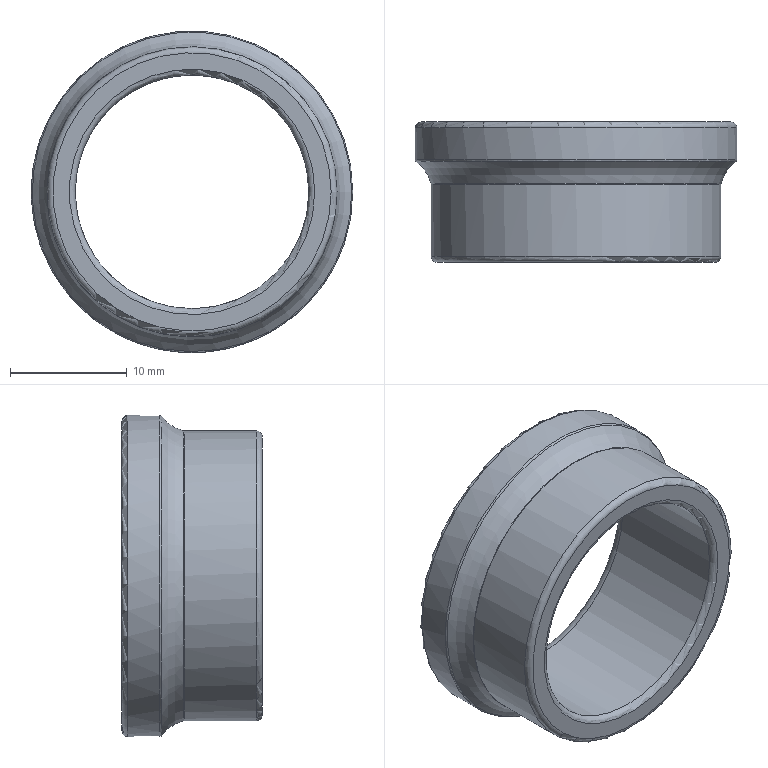Part | STEP file | BK-20_id1254_x_t | 1 solid | 12 faces | box 27.5 x 12 x 27.5 mm | volume 2449 mm3 | torus 7 | cylinder 3 | plane 2 | commonest cylinder face diameters 20 x1 24.8 x1 27.5 x1
STEP:
#1=CARTESIAN_POINT('',(0.,0.,0.));
#2=DIRECTION('',(0.,0.,1.));
#3=DIRECTION('',(1.,0.,0.));
#4=AXIS2_PLACEMENT_3D('',#1,#2,#3);
#5=CARTESIAN_POINT('',(-260.083,526.527,-176.266));
#6=VERTEX_POINT('',#5);
#7=CARTESIAN_POINT('',(-254.834,526.527,-165.5));
#8=VERTEX_POINT('',#7);
#9=CARTESIAN_POINT('',(-268.5,526.527,-165.5));
#10=DIRECTION('',(0.,1.,0.));
#11=DIRECTION('',(0.6159,0.,-0.7878));
#12=AXIS2_PLACEMENT_3D('',#9,#10,#11);
#13=CIRCLE('',#12,13.666);
#14=CARTESIAN_POINT('',(-268.5,523.936,-165.5));
#15=DIRECTION('',(0.,-1.,0.));
#16=DIRECTION('',(1.,0.,0.));
#17=AXIS2_PLACEMENT_3D('',#14,#15,#16);
#18=TOROIDAL_SURFACE('',#17,15.5,3.175);
#19=CARTESIAN_POINT('',(11.659,4.096));
#20=DIRECTION('',(-1.,0.));
#21=VECTOR('',#20,1.);
#22=LINE('',#19,#21);
#23=(GEOMETRIC_REPRESENTATION_CONTEXT(2)PARAMETRIC_REPRESENTATION_CONTEXT()REPRESENTATION_CONTEXT('',''));
#24=DEFINITIONAL_REPRESENTATION('',(#22),#23);
#25=PCURVE('',#18,#24);
#26=CARTESIAN_POINT('',(-268.5,526.69,-165.5));
#27=DIRECTION('',(0.,-1.,0.));
#28=DIRECTION('',(1.,0.,0.));
#29=AXIS2_PLACEMENT_3D('',#26,#27,#28);
#30=TOROIDAL_SURFACE('',#29,13.55,0.2);
#31=CARTESIAN_POINT('',(5.376,7.238));
#32=DIRECTION('',(-1.,0.));
#33=VECTOR('',#32,1.);
#34=LINE('',#31,#33);
#35=(GEOMETRIC_REPRESENTATION_CONTEXT(2)PARAMETRIC_REPRESENTATION_CONTEXT()REPRESENTATION_CONTEXT('',''));
#36=DEFINITIONAL_REPRESENTATION('',(#34),#35);
#37=PCURVE('',#30,#36);
#38=SURFACE_CURVE('',#13,(#25,#37),.PCURVE_S1.);
#39=EDGE_CURVE('',#6,#8,#38,.T.);
#40=ORIENTED_EDGE('',*,*,#39,.T.);
#41=CARTESIAN_POINT('',(-268.5,526.527,-165.5));
#42=DIRECTION('',(0.,1.,0.));
#43=DIRECTION('',(0.6159,0.,-0.7878));
#44=AXIS2_PLACEMENT_3D('',#41,#42,#43);
#45=CIRCLE('',#44,13.666);
#46=CARTESIAN_POINT('',(11.659,4.096));
#47=DIRECTION('',(-1.,0.));
#48=VECTOR('',#47,1.);
#49=LINE('',#46,#48);
#50=(GEOMETRIC_REPRESENTATION_CONTEXT(2)PARAMETRIC_REPRESENTATION_CONTEXT()REPRESENTATION_CONTEXT('',''));
#51=DEFINITIONAL_REPRESENTATION('',(#49),#50);
#52=PCURVE('',#18,#51);
#53=CARTESIAN_POINT('',(11.659,7.238));
#54=DIRECTION('',(-1.,0.));
#55=VECTOR('',#54,1.);
#56=LINE('',#53,#55);
#57=(GEOMETRIC_REPRESENTATION_CONTEXT(2)PARAMETRIC_REPRESENTATION_CONTEXT()REPRESENTATION_CONTEXT('',''));
#58=DEFINITIONAL_REPRESENTATION('',(#56),#57);
#59=PCURVE('',#30,#58);
#60=SURFACE_CURVE('',#45,(#52,#59),.PCURVE_S1.);
#61=EDGE_CURVE('',#8,#6,#60,.T.);
#62=ORIENTED_EDGE('',*,*,#61,.T.);
#63=CARTESIAN_POINT('',(-260.86,524.644,-175.273));
#64=VERTEX_POINT('',#63);
#65=CARTESIAN_POINT('',(-260.86,524.644,-175.273));
#66=CARTESIAN_POINT('',(-260.806,525.022,-175.341));
#67=CARTESIAN_POINT('',(-260.719,525.386,-175.453));
#68=CARTESIAN_POINT('',(-260.6,525.725,-175.605));
#69=CARTESIAN_POINT('',(-260.452,526.034,-175.794));
#70=CARTESIAN_POINT('',(-260.278,526.303,-176.017));
#71=CARTESIAN_POINT('',(-260.083,526.527,-176.266));
#72=(BOUNDED_CURVE()B_SPLINE_CURVE(6,(#65,#66,#67,#68,#69,#70,#71),.UNSPECIFIED.,.F.,.F.)B_SPLINE_CURVE_WITH_KNOTS((7,7),(3.367,4.096),.PIECEWISE_BEZIER_KNOTS.)CURVE()GEOMETRIC_REPRESENTATION_ITEM()RATIONAL_B_SPLINE_CURVE((1.007,1.002,0.9996,0.9987,0.9996,1.002,1.007))REPRESENTATION_ITEM(''));
#73=CARTESIAN_POINT('',(5.376,0.));
#74=DIRECTION('',(0.,1.));
#75=VECTOR('',#74,1.);
#76=LINE('',#73,#75);
#77=(GEOMETRIC_REPRESENTATION_CONTEXT(2)PARAMETRIC_REPRESENTATION_CONTEXT()REPRESENTATION_CONTEXT('',''));
#78=DEFINITIONAL_REPRESENTATION('',(#76),#77);
#79=PCURVE('',#18,#78);
#80=CARTESIAN_POINT('',(11.659,0.));
#81=DIRECTION('',(0.,1.));
#82=VECTOR('',#81,1.);
#83=LINE('',#80,#82);
#84=(GEOMETRIC_REPRESENTATION_CONTEXT(2)PARAMETRIC_REPRESENTATION_CONTEXT()REPRESENTATION_CONTEXT('',''));
#85=DEFINITIONAL_REPRESENTATION('',(#83),#84);
#86=PCURVE('',#18,#85);
#87=SEAM_CURVE('',#72,(#79,#86),.PCURVE_S1.);
#88=EDGE_CURVE('',#64,#6,#87,.T.);
#89=ORIENTED_EDGE('',*,*,#88,.F.);
#90=CARTESIAN_POINT('',(-256.095,524.644,-165.5));
#91=VERTEX_POINT('',#90);
#92=CARTESIAN_POINT('',(-268.5,524.644,-165.5));
#93=DIRECTION('',(0.,1.,0.));
#94=DIRECTION('',(-0.6159,0.,0.7878));
#95=AXIS2_PLACEMENT_3D('',#92,#93,#94);
#96=CIRCLE('',#95,12.405);
#97=CARTESIAN_POINT('',(8.518,3.367));
#98=DIRECTION('',(-1.,0.));
#99=VECTOR('',#98,1.);
#100=LINE('',#97,#99);
#101=(GEOMETRIC_REPRESENTATION_CONTEXT(2)PARAMETRIC_REPRESENTATION_CONTEXT()REPRESENTATION_CONTEXT('',''));
#102=DEFINITIONAL_REPRESENTATION('',(#100),#101);
#103=PCURVE('',#18,#102);
#104=CARTESIAN_POINT('',(-268.5,524.599,-165.5));
#105=DIRECTION('',(0.,-1.,0.));
#106=DIRECTION('',(1.,0.,0.));
#107=AXIS2_PLACEMENT_3D('',#104,#105,#106);
#108=TOROIDAL_SURFACE('',#107,12.6,0.2);
#109=CARTESIAN_POINT('',(8.518,3.367));
#110=DIRECTION('',(-1.,0.));
#111=VECTOR('',#110,1.);
#112=LINE('',#109,#111);
#113=(GEOMETRIC_REPRESENTATION_CONTEXT(2)PARAMETRIC_REPRESENTATION_CONTEXT()REPRESENTATION_CONTEXT('',''));
#114=DEFINITIONAL_REPRESENTATION('',(#112),#113);
#115=PCURVE('',#108,#114);
#116=SURFACE_CURVE('',#96,(#103,#115),.PCURVE_S1.);
#117=EDGE_CURVE('',#91,#64,#116,.T.);
#118=ORIENTED_EDGE('',*,*,#117,.F.);
#119=CARTESIAN_POINT('',(-276.14,524.644,-155.727));
#120=VERTEX_POINT('',#119);
#121=CARTESIAN_POINT('',(-268.5,524.644,-165.5));
#122=DIRECTION('',(0.,1.,0.));
#123=DIRECTION('',(-0.6159,0.,0.7878));
#124=AXIS2_PLACEMENT_3D('',#121,#122,#123);
#125=CIRCLE('',#124,12.405);
#126=CARTESIAN_POINT('',(8.518,3.367));
#127=DIRECTION('',(-1.,0.));
#128=VECTOR('',#127,1.);
#129=LINE('',#126,#128);
#130=(GEOMETRIC_REPRESENTATION_CONTEXT(2)PARAMETRIC_REPRESENTATION_CONTEXT()REPRESENTATION_CONTEXT('',''));
#131=DEFINITIONAL_REPRESENTATION('',(#129),#130);
#132=PCURVE('',#18,#131);
#133=CARTESIAN_POINT('',(2.234,3.367));
#134=DIRECTION('',(-1.,0.));
#135=VECTOR('',#134,1.);
#136=LINE('',#133,#135);
#137=(GEOMETRIC_REPRESENTATION_CONTEXT(2)PARAMETRIC_REPRESENTATION_CONTEXT()REPRESENTATION_CONTEXT('',''));
#138=DEFINITIONAL_REPRESENTATION('',(#136),#137);
#139=PCURVE('',#108,#138);
#140=SURFACE_CURVE('',#125,(#132,#139),.PCURVE_S1.);
#141=EDGE_CURVE('',#120,#91,#140,.T.);
#142=ORIENTED_EDGE('',*,*,#141,.F.);
#143=CARTESIAN_POINT('',(-268.5,524.644,-165.5));
#144=DIRECTION('',(0.,1.,0.));
#145=DIRECTION('',(-0.6159,0.,0.7878));
#146=AXIS2_PLACEMENT_3D('',#143,#144,#145);
#147=CIRCLE('',#146,12.405);
#148=CARTESIAN_POINT('',(14.801,3.367));
#149=DIRECTION('',(-1.,0.));
#150=VECTOR('',#149,1.);
#151=LINE('',#148,#150);
#152=(GEOMETRIC_REPRESENTATION_CONTEXT(2)PARAMETRIC_REPRESENTATION_CONTEXT()REPRESENTATION_CONTEXT('',''));
#153=DEFINITIONAL_REPRESENTATION('',(#151),#152);
#154=PCURVE('',#18,#153);
#155=CARTESIAN_POINT('',(8.518,3.367));
#156=DIRECTION('',(-1.,0.));
#157=VECTOR('',#156,1.);
#158=LINE('',#155,#157);
#159=(GEOMETRIC_REPRESENTATION_CONTEXT(2)PARAMETRIC_REPRESENTATION_CONTEXT()REPRESENTATION_CONTEXT('',''));
#160=DEFINITIONAL_REPRESENTATION('',(#158),#159);
#161=PCURVE('',#108,#160);
#162=SURFACE_CURVE('',#147,(#154,#161),.PCURVE_S1.);
#163=EDGE_CURVE('',#64,#120,#162,.T.);
#164=ORIENTED_EDGE('',*,*,#163,.F.);
#165=ORIENTED_EDGE('',*,*,#88,.T.);
#166=EDGE_LOOP('',(#40,#62,#89,#118,#142,#164,#165));
#167=FACE_BOUND('',#166,.F.);
#168=ADVANCED_FACE('',(#167),#18,.F.);
#169=CARTESIAN_POINT('',(-256.1,524.599,-165.5));
#170=VERTEX_POINT('',#169);
#171=CARTESIAN_POINT('',(-268.5,524.599,-165.5));
#172=DIRECTION('',(0.,-1.,0.));
#173=DIRECTION('',(1.,0.,0.));
#174=AXIS2_PLACEMENT_3D('',#171,#172,#173);
#175=CIRCLE('',#174,12.4);
#176=CARTESIAN_POINT('',(0.,3.142));
#177=DIRECTION('',(1.,0.));
#178=VECTOR('',#177,1.);
#179=LINE('',#176,#178);
#180=(GEOMETRIC_REPRESENTATION_CONTEXT(2)PARAMETRIC_REPRESENTATION_CONTEXT()REPRESENTATION_CONTEXT('',''));
#181=DEFINITIONAL_REPRESENTATION('',(#179),#180);
#182=PCURVE('',#108,#181);
#183=CARTESIAN_POINT('',(-268.5,493.093,-165.5));
#184=DIRECTION('',(0.,-1.,0.));
#185=DIRECTION('',(1.,0.,0.));
#186=AXIS2_PLACEMENT_3D('',#183,#184,#185);
#187=CYLINDRICAL_SURFACE('',#186,12.4);
#188=CARTESIAN_POINT('',(0.,-31.507));
#189=DIRECTION('',(1.,0.));
#190=VECTOR('',#189,1.);
#191=LINE('',#188,#190);
#192=(GEOMETRIC_REPRESENTATION_CONTEXT(2)PARAMETRIC_REPRESENTATION_CONTEXT()REPRESENTATION_CONTEXT('',''));
#193=DEFINITIONAL_REPRESENTATION('',(#191),#192);
#194=PCURVE('',#187,#193);
#195=SURFACE_CURVE('',#175,(#182,#194),.PCURVE_S1.);
#196=EDGE_CURVE('',#170,#170,#195,.T.);
#197=ORIENTED_EDGE('',*,*,#196,.T.);
#198=CARTESIAN_POINT('',(-256.1,524.599,-165.5));
#199=CARTESIAN_POINT('',(-256.1,524.607,-165.5));
#200=CARTESIAN_POINT('',(-256.1,524.614,-165.5));
#201=CARTESIAN_POINT('',(-256.099,524.622,-165.5));
#202=CARTESIAN_POINT('',(-256.098,524.629,-165.5));
#203=CARTESIAN_POINT('',(-256.097,524.637,-165.5));
#204=CARTESIAN_POINT('',(-256.095,524.644,-165.5));
#205=(BOUNDED_CURVE()B_SPLINE_CURVE(6,(#198,#199,#200,#201,#202,#203,#204),.UNSPECIFIED.,.F.,.F.)B_SPLINE_CURVE_WITH_KNOTS((7,7),(3.142,3.367),.PIECEWISE_BEZIER_KNOTS.)CURVE()GEOMETRIC_REPRESENTATION_ITEM()RATIONAL_B_SPLINE_CURVE((1.001,1.,1.,0.9999,1.,1.,1.001))REPRESENTATION_ITEM(''));
#206=CARTESIAN_POINT('',(6.283,0.));
#207=DIRECTION('',(0.,1.));
#208=VECTOR('',#207,1.);
#209=LINE('',#206,#208);
#210=(GEOMETRIC_REPRESENTATION_CONTEXT(2)PARAMETRIC_REPRESENTATION_CONTEXT()REPRESENTATION_CONTEXT('',''));
#211=DEFINITIONAL_REPRESENTATION('',(#209),#210);
#212=PCURVE('',#108,#211);
#213=CARTESIAN_POINT('',(0.,0.));
#214=DIRECTION('',(0.,1.));
#215=VECTOR('',#214,1.);
#216=LINE('',#213,#215);
#217=(GEOMETRIC_REPRESENTATION_CONTEXT(2)PARAMETRIC_REPRESENTATION_CONTEXT()REPRESENTATION_CONTEXT('',''));
#218=DEFINITIONAL_REPRESENTATION('',(#216),#217);
#219=PCURVE('',#108,#218);
#220=SEAM_CURVE('',#205,(#212,#219),.PCURVE_S1.);
#221=EDGE_CURVE('',#170,#91,#220,.T.);
#222=ORIENTED_EDGE('',*,*,#221,.T.);
#223=ORIENTED_EDGE('',*,*,#117,.T.);
#224=ORIENTED_EDGE('',*,*,#163,.T.);
#225=ORIENTED_EDGE('',*,*,#141,.T.);
#226=ORIENTED_EDGE('',*,*,#221,.F.);
#227=EDGE_LOOP('',(#197,#222,#223,#224,#225,#226));
#228=FACE_BOUND('',#227,.F.);
#229=ADVANCED_FACE('',(#228),#108,.F.);
#230=CARTESIAN_POINT('',(-254.75,526.69,-165.5));
#231=VERTEX_POINT('',#230);
#232=CARTESIAN_POINT('',(-268.5,526.69,-165.5));
#233=DIRECTION('',(0.,1.,0.));
#234=DIRECTION('',(1.,0.,0.));
#235=AXIS2_PLACEMENT_3D('',#232,#233,#234);
#236=CIRCLE('',#235,13.75);
#237=CARTESIAN_POINT('',(6.283,6.283));
#238=DIRECTION('',(-1.,0.));
#239=VECTOR('',#238,1.);
#240=LINE('',#237,#239);
#241=(GEOMETRIC_REPRESENTATION_CONTEXT(2)PARAMETRIC_REPRESENTATION_CONTEXT()REPRESENTATION_CONTEXT('',''));
#242=DEFINITIONAL_REPRESENTATION('',(#240),#241);
#243=PCURVE('',#30,#242);
#244=CARTESIAN_POINT('',(-268.5,493.093,-165.5));
#245=DIRECTION('',(0.,-1.,0.));
#246=DIRECTION('',(1.,0.,0.));
#247=AXIS2_PLACEMENT_3D('',#244,#245,#246);
#248=CYLINDRICAL_SURFACE('',#247,13.75);
#249=CARTESIAN_POINT('',(6.283,-33.598));
#250=DIRECTION('',(-1.,0.));
#251=VECTOR('',#250,1.);
#252=LINE('',#249,#251);
#253=(GEOMETRIC_REPRESENTATION_CONTEXT(2)PARAMETRIC_REPRESENTATION_CONTEXT()REPRESENTATION_CONTEXT('',''));
#254=DEFINITIONAL_REPRESENTATION('',(#252),#253);
#255=PCURVE('',#248,#254);
#256=SURFACE_CURVE('',#236,(#243,#255),.PCURVE_S1.);
#257=EDGE_CURVE('',#231,#231,#256,.T.);
#258=ORIENTED_EDGE('',*,*,#257,.F.);
#259=CARTESIAN_POINT('',(-254.75,526.69,-165.5));
#260=CARTESIAN_POINT('',(-254.75,526.658,-165.5));
#261=CARTESIAN_POINT('',(-254.756,526.626,-165.5));
#262=CARTESIAN_POINT('',(-254.768,526.596,-165.5));
#263=CARTESIAN_POINT('',(-254.786,526.569,-165.5));
#264=CARTESIAN_POINT('',(-254.808,526.546,-165.5));
#265=CARTESIAN_POINT('',(-254.834,526.527,-165.5));
#266=(BOUNDED_CURVE()B_SPLINE_CURVE(6,(#259,#260,#261,#262,#263,#264,#265),.UNSPECIFIED.,.F.,.F.)B_SPLINE_CURVE_WITH_KNOTS((7,7),(0.,0.9548),.PIECEWISE_BEZIER_KNOTS.)CURVE()GEOMETRIC_REPRESENTATION_ITEM()RATIONAL_B_SPLINE_CURVE((1.011,1.004,0.9992,0.9977,0.9992,1.004,1.011))REPRESENTATION_ITEM(''));
#267=CARTESIAN_POINT('',(6.283,6.283));
#268=DIRECTION('',(0.,1.));
#269=VECTOR('',#268,1.);
#270=LINE('',#267,#269);
#271=(GEOMETRIC_REPRESENTATION_CONTEXT(2)PARAMETRIC_REPRESENTATION_CONTEXT()REPRESENTATION_CONTEXT('',''));
#272=DEFINITIONAL_REPRESENTATION('',(#270),#271);
#273=PCURVE('',#30,#272);
#274=CARTESIAN_POINT('',(0.,6.283));
#275=DIRECTION('',(0.,1.));
#276=VECTOR('',#275,1.);
#277=LINE('',#274,#276);
#278=(GEOMETRIC_REPRESENTATION_CONTEXT(2)PARAMETRIC_REPRESENTATION_CONTEXT()REPRESENTATION_CONTEXT('',''));
#279=DEFINITIONAL_REPRESENTATION('',(#277),#278);
#280=PCURVE('',#30,#279);
#281=SEAM_CURVE('',#266,(#273,#280),.PCURVE_S1.);
#282=EDGE_CURVE('',#231,#8,#281,.T.);
#283=ORIENTED_EDGE('',*,*,#282,.T.);
#284=ORIENTED_EDGE('',*,*,#61,.T.);
#285=ORIENTED_EDGE('',*,*,#39,.T.);
#286=ORIENTED_EDGE('',*,*,#282,.F.);
#287=EDGE_LOOP('',(#258,#283,#284,#285,#286));
#288=FACE_BOUND('',#287,.T.);
#289=ADVANCED_FACE('',(#288),#30,.T.);
#290=CARTESIAN_POINT('',(-256.1,518.436,-165.5));
#291=VERTEX_POINT('',#290);
#292=CARTESIAN_POINT('',(-260.863,518.436,-175.269));
#293=VERTEX_POINT('',#292);
#294=CARTESIAN_POINT('',(-268.5,518.436,-165.5));
#295=DIRECTION('',(0.,-1.,0.));
#296=DIRECTION('',(0.6159,0.,-0.7878));
#297=AXIS2_PLACEMENT_3D('',#294,#295,#296);
#298=CIRCLE('',#297,12.4);
#299=CARTESIAN_POINT('',(-0.9073,-25.343));
#300=DIRECTION('',(1.,0.));
#301=VECTOR('',#300,1.);
#302=LINE('',#299,#301);
#303=(GEOMETRIC_REPRESENTATION_CONTEXT(2)PARAMETRIC_REPRESENTATION_CONTEXT()REPRESENTATION_CONTEXT('',''));
#304=DEFINITIONAL_REPRESENTATION('',(#302),#303);
#305=PCURVE('',#187,#304);
#306=CARTESIAN_POINT('',(-268.5,518.436,-165.5));
#307=DIRECTION('',(0.,-1.,0.));
#308=DIRECTION('',(1.,0.,0.));
#309=AXIS2_PLACEMENT_3D('',#306,#307,#308);
#310=TOROIDAL_SURFACE('',#309,11.9,0.5);
#311=CARTESIAN_POINT('',(-0.9073,6.283));
#312=DIRECTION('',(1.,0.));
#313=VECTOR('',#312,1.);
#314=LINE('',#311,#313);
#315=(GEOMETRIC_REPRESENTATION_CONTEXT(2)PARAMETRIC_REPRESENTATION_CONTEXT()REPRESENTATION_CONTEXT('',''));
#316=DEFINITIONAL_REPRESENTATION('',(#314),#315);
#317=PCURVE('',#310,#316);
#318=SURFACE_CURVE('',#298,(#305,#317),.PCURVE_S1.);
#319=EDGE_CURVE('',#291,#293,#318,.T.);
#320=ORIENTED_EDGE('',*,*,#319,.F.);
#321=CARTESIAN_POINT('',(-256.1,524.599,-165.5));
#322=CARTESIAN_POINT('',(-256.1,518.436,-165.5));
#323=B_SPLINE_CURVE_WITH_KNOTS('',1,(#321,#322),.UNSPECIFIED.,.F.,.F.,(2,2),(-31.507,-25.343),.PIECEWISE_BEZIER_KNOTS.);
#324=CARTESIAN_POINT('',(0.,0.));
#325=DIRECTION('',(0.,1.));
#326=VECTOR('',#325,1.);
#327=LINE('',#324,#326);
#328=(GEOMETRIC_REPRESENTATION_CONTEXT(2)PARAMETRIC_REPRESENTATION_CONTEXT()REPRESENTATION_CONTEXT('',''));
#329=DEFINITIONAL_REPRESENTATION('',(#327),#328);
#330=PCURVE('',#187,#329);
#331=CARTESIAN_POINT('',(6.283,0.));
#332=DIRECTION('',(0.,1.));
#333=VECTOR('',#332,1.);
#334=LINE('',#331,#333);
#335=(GEOMETRIC_REPRESENTATION_CONTEXT(2)PARAMETRIC_REPRESENTATION_CONTEXT()REPRESENTATION_CONTEXT('',''));
#336=DEFINITIONAL_REPRESENTATION('',(#334),#335);
#337=PCURVE('',#187,#336);
#338=SEAM_CURVE('',#323,(#330,#337),.PCURVE_S1.);
#339=EDGE_CURVE('',#170,#291,#338,.T.);
#340=ORIENTED_EDGE('',*,*,#339,.F.);
#341=ORIENTED_EDGE('',*,*,#196,.T.);
#342=ORIENTED_EDGE('',*,*,#339,.T.);
#343=CARTESIAN_POINT('',(-268.5,518.436,-165.5));
#344=DIRECTION('',(0.,-1.,0.));
#345=DIRECTION('',(0.6159,0.,-0.7878));
#346=AXIS2_PLACEMENT_3D('',#343,#344,#345);
#347=CIRCLE('',#346,12.4);
#348=CARTESIAN_POINT('',(5.376,-25.343));
#349=DIRECTION('',(1.,0.));
#350=VECTOR('',#349,1.);
#351=LINE('',#348,#350);
#352=(GEOMETRIC_REPRESENTATION_CONTEXT(2)PARAMETRIC_REPRESENTATION_CONTEXT()REPRESENTATION_CONTEXT('',''));
#353=DEFINITIONAL_REPRESENTATION('',(#351),#352);
#354=PCURVE('',#187,#353);
#355=CARTESIAN_POINT('',(5.376,6.283));
#356=DIRECTION('',(1.,0.));
#357=VECTOR('',#356,1.);
#358=LINE('',#355,#357);
#359=(GEOMETRIC_REPRESENTATION_CONTEXT(2)PARAMETRIC_REPRESENTATION_CONTEXT()REPRESENTATION_CONTEXT('',''));
#360=DEFINITIONAL_REPRESENTATION('',(#358),#359);
#361=PCURVE('',#310,#360);
#362=SURFACE_CURVE('',#347,(#354,#361),.PCURVE_S1.);
#363=EDGE_CURVE('',#293,#291,#362,.T.);
#364=ORIENTED_EDGE('',*,*,#363,.F.);
#365=EDGE_LOOP('',(#320,#340,#341,#342,#364));
#366=FACE_BOUND('',#365,.T.);
#367=ADVANCED_FACE('',(#366),#187,.T.);
#368=ORIENTED_EDGE('',*,*,#257,.T.);
#369=CARTESIAN_POINT('',(-254.75,529.436,-165.5));
#370=VERTEX_POINT('',#369);
#371=CARTESIAN_POINT('',(-254.75,529.436,-165.5));
#372=CARTESIAN_POINT('',(-254.75,526.69,-165.5));
#373=B_SPLINE_CURVE_WITH_KNOTS('',1,(#371,#372),.UNSPECIFIED.,.F.,.F.,(2,2),(-36.343,-33.598),.PIECEWISE_BEZIER_KNOTS.);
#374=CARTESIAN_POINT('',(0.,0.));
#375=DIRECTION('',(0.,1.));
#376=VECTOR('',#375,1.);
#377=LINE('',#374,#376);
#378=(GEOMETRIC_REPRESENTATION_CONTEXT(2)PARAMETRIC_REPRESENTATION_CONTEXT()REPRESENTATION_CONTEXT('',''));
#379=DEFINITIONAL_REPRESENTATION('',(#377),#378);
#380=PCURVE('',#248,#379);
#381=CARTESIAN_POINT('',(6.283,0.));
#382=DIRECTION('',(0.,1.));
#383=VECTOR('',#382,1.);
#384=LINE('',#381,#383);
#385=(GEOMETRIC_REPRESENTATION_CONTEXT(2)PARAMETRIC_REPRESENTATION_CONTEXT()REPRESENTATION_CONTEXT('',''));
#386=DEFINITIONAL_REPRESENTATION('',(#384),#385);
#387=PCURVE('',#248,#386);
#388=SEAM_CURVE('',#373,(#380,#387),.PCURVE_S1.);
#389=EDGE_CURVE('',#370,#231,#388,.T.);
#390=ORIENTED_EDGE('',*,*,#389,.F.);
#391=CARTESIAN_POINT('',(-260.031,529.436,-176.333));
#392=VERTEX_POINT('',#391);
#393=CARTESIAN_POINT('',(-268.5,529.436,-165.5));
#394=DIRECTION('',(0.,1.,0.));
#395=DIRECTION('',(0.6159,0.,-0.7878));
#396=AXIS2_PLACEMENT_3D('',#393,#394,#395);
#397=CIRCLE('',#396,13.75);
#398=CARTESIAN_POINT('',(5.376,-36.343));
#399=DIRECTION('',(-1.,0.));
#400=VECTOR('',#399,1.);
#401=LINE('',#398,#400);
#402=(GEOMETRIC_REPRESENTATION_CONTEXT(2)PARAMETRIC_REPRESENTATION_CONTEXT()REPRESENTATION_CONTEXT('',''));
#403=DEFINITIONAL_REPRESENTATION('',(#401),#402);
#404=PCURVE('',#248,#403);
#405=CARTESIAN_POINT('',(-268.5,529.436,-165.5));
#406=DIRECTION('',(0.,-1.,0.));
#407=DIRECTION('',(1.,0.,0.));
#408=AXIS2_PLACEMENT_3D('',#405,#406,#407);
#409=TOROIDAL_SURFACE('',#408,13.25,0.5);
#410=CARTESIAN_POINT('',(5.376,6.283));
#411=DIRECTION('',(-1.,0.));
#412=VECTOR('',#411,1.);
#413=LINE('',#410,#412);
#414=(GEOMETRIC_REPRESENTATION_CONTEXT(2)PARAMETRIC_REPRESENTATION_CONTEXT()REPRESENTATION_CONTEXT('',''));
#415=DEFINITIONAL_REPRESENTATION('',(#413),#414);
#416=PCURVE('',#409,#415);
#417=SURFACE_CURVE('',#397,(#404,#416),.PCURVE_S1.);
#418=EDGE_CURVE('',#392,#370,#417,.T.);
#419=ORIENTED_EDGE('',*,*,#418,.F.);
#420=CARTESIAN_POINT('',(-268.5,529.436,-165.5));
#421=DIRECTION('',(0.,1.,0.));
#422=DIRECTION('',(0.6159,0.,-0.7878));
#423=AXIS2_PLACEMENT_3D('',#420,#421,#422);
#424=CIRCLE('',#423,13.75);
#425=CARTESIAN_POINT('',(11.659,-36.343));
#426=DIRECTION('',(-1.,0.));
#427=VECTOR('',#426,1.);
#428=LINE('',#425,#427);
#429=(GEOMETRIC_REPRESENTATION_CONTEXT(2)PARAMETRIC_REPRESENTATION_CONTEXT()REPRESENTATION_CONTEXT('',''));
#430=DEFINITIONAL_REPRESENTATION('',(#428),#429);
#431=PCURVE('',#248,#430);
#432=CARTESIAN_POINT('',(11.659,6.283));
#433=DIRECTION('',(-1.,0.));
#434=VECTOR('',#433,1.);
#435=LINE('',#432,#434);
#436=(GEOMETRIC_REPRESENTATION_CONTEXT(2)PARAMETRIC_REPRESENTATION_CONTEXT()REPRESENTATION_CONTEXT('',''));
#437=DEFINITIONAL_REPRESENTATION('',(#435),#436);
#438=PCURVE('',#409,#437);
#439=SURFACE_CURVE('',#424,(#431,#438),.PCURVE_S1.);
#440=EDGE_CURVE('',#370,#392,#439,.T.);
#441=ORIENTED_EDGE('',*,*,#440,.F.);
#442=ORIENTED_EDGE('',*,*,#389,.T.);
#443=EDGE_LOOP('',(#368,#390,#419,#441,#442));
#444=FACE_BOUND('',#443,.T.);
#445=ADVANCED_FACE('',(#444),#248,.T.);
#446=ORIENTED_EDGE('',*,*,#363,.T.);
#447=CARTESIAN_POINT('',(-256.6,517.936,-165.5));
#448=VERTEX_POINT('',#447);
#449=CARTESIAN_POINT('',(-256.1,518.436,-165.5));
#450=CARTESIAN_POINT('',(-256.1,518.302,-165.5));
#451=CARTESIAN_POINT('',(-256.143,518.172,-165.5));
#452=CARTESIAN_POINT('',(-256.224,518.06,-165.5));
#453=CARTESIAN_POINT('',(-256.336,517.978,-165.5));
#454=CARTESIAN_POINT('',(-256.466,517.936,-165.5));
#455=CARTESIAN_POINT('',(-256.6,517.936,-165.5));
#456=(BOUNDED_CURVE()B_SPLINE_CURVE(6,(#449,#450,#451,#452,#453,#454,#455),.UNSPECIFIED.,.F.,.F.)B_SPLINE_CURVE_WITH_KNOTS((7,7),(0.,1.571),.PIECEWISE_BEZIER_KNOTS.)CURVE()GEOMETRIC_REPRESENTATION_ITEM()RATIONAL_B_SPLINE_CURVE((1.031,1.01,0.9979,0.994,0.9979,1.01,1.031))REPRESENTATION_ITEM(''));
#457=CARTESIAN_POINT('',(6.283,6.283));
#458=DIRECTION('',(0.,1.));
#459=VECTOR('',#458,1.);
#460=LINE('',#457,#459);
#461=(GEOMETRIC_REPRESENTATION_CONTEXT(2)PARAMETRIC_REPRESENTATION_CONTEXT()REPRESENTATION_CONTEXT('',''));
#462=DEFINITIONAL_REPRESENTATION('',(#460),#461);
#463=PCURVE('',#310,#462);
#464=CARTESIAN_POINT('',(0.,6.283));
#465=DIRECTION('',(0.,1.));
#466=VECTOR('',#465,1.);
#467=LINE('',#464,#466);
#468=(GEOMETRIC_REPRESENTATION_CONTEXT(2)PARAMETRIC_REPRESENTATION_CONTEXT()REPRESENTATION_CONTEXT('',''));
#469=DEFINITIONAL_REPRESENTATION('',(#467),#468);
#470=PCURVE('',#310,#469);
#471=SEAM_CURVE('',#456,(#463,#470),.PCURVE_S1.);
#472=EDGE_CURVE('',#291,#448,#471,.T.);
#473=ORIENTED_EDGE('',*,*,#472,.T.);
#474=CARTESIAN_POINT('',(-268.5,517.936,-165.5));
#475=DIRECTION('',(0.,1.,0.));
#476=DIRECTION('',(1.,0.,0.));
#477=AXIS2_PLACEMENT_3D('',#474,#475,#476);
#478=CIRCLE('',#477,11.9);
#479=CARTESIAN_POINT('',(6.283,7.854));
#480=DIRECTION('',(-1.,0.));
#481=VECTOR('',#480,1.);
#482=LINE('',#479,#481);
#483=(GEOMETRIC_REPRESENTATION_CONTEXT(2)PARAMETRIC_REPRESENTATION_CONTEXT()REPRESENTATION_CONTEXT('',''));
#484=DEFINITIONAL_REPRESENTATION('',(#482),#483);
#485=PCURVE('',#310,#484);
#486=CARTESIAN_POINT('',(-276.772,517.936,-171.967));
#487=DIRECTION('',(0.,1.,0.));
#488=DIRECTION('',(-1.,0.,0.));
#489=AXIS2_PLACEMENT_3D('',#486,#487,#488);
#490=PLANE('',#489);
#491=CARTESIAN_POINT('',(-8.272,6.467));
#492=DIRECTION('',(-1.,0.));
#493=AXIS2_PLACEMENT_2D('',#491,#492);
#494=CIRCLE('',#493,11.9);
#495=(GEOMETRIC_REPRESENTATION_CONTEXT(2)PARAMETRIC_REPRESENTATION_CONTEXT()REPRESENTATION_CONTEXT('',''));
#496=DEFINITIONAL_REPRESENTATION('',(#494),#495);
#497=PCURVE('',#490,#496);
#498=SURFACE_CURVE('',#478,(#485,#497),.PCURVE_S1.);
#499=EDGE_CURVE('',#448,#448,#498,.T.);
#500=ORIENTED_EDGE('',*,*,#499,.T.);
#501=ORIENTED_EDGE('',*,*,#472,.F.);
#502=ORIENTED_EDGE('',*,*,#319,.T.);
#503=EDGE_LOOP('',(#446,#473,#500,#501,#502));
#504=FACE_BOUND('',#503,.T.);
#505=ADVANCED_FACE('',(#504),#310,.T.);
#506=CARTESIAN_POINT('',(-255.25,529.936,-165.5));
#507=VERTEX_POINT('',#506);
#508=CARTESIAN_POINT('',(-268.5,529.936,-165.5));
#509=DIRECTION('',(0.,-1.,0.));
#510=DIRECTION('',(1.,0.,0.));
#511=AXIS2_PLACEMENT_3D('',#508,#509,#510);
#512=CIRCLE('',#511,13.25);
#513=CARTESIAN_POINT('',(0.,4.712));
#514=DIRECTION('',(1.,0.));
#515=VECTOR('',#514,1.);
#516=LINE('',#513,#515);
#517=(GEOMETRIC_REPRESENTATION_CONTEXT(2)PARAMETRIC_REPRESENTATION_CONTEXT()REPRESENTATION_CONTEXT('',''));
#518=DEFINITIONAL_REPRESENTATION('',(#516),#517);
#519=PCURVE('',#409,#518);
#520=CARTESIAN_POINT('',(-277.166,529.936,-172.275));
#521=DIRECTION('',(0.,-1.,0.));
#522=DIRECTION('',(1.,0.,0.));
#523=AXIS2_PLACEMENT_3D('',#520,#521,#522);
#524=PLANE('',#523);
#525=CARTESIAN_POINT('',(8.666,6.775));
#526=DIRECTION('',(1.,0.));
#527=AXIS2_PLACEMENT_2D('',#525,#526);
#528=CIRCLE('',#527,13.25);
#529=(GEOMETRIC_REPRESENTATION_CONTEXT(2)PARAMETRIC_REPRESENTATION_CONTEXT()REPRESENTATION_CONTEXT('',''));
#530=DEFINITIONAL_REPRESENTATION('',(#528),#529);
#531=PCURVE('',#524,#530);
#532=SURFACE_CURVE('',#512,(#519,#531),.PCURVE_S1.);
#533=EDGE_CURVE('',#507,#507,#532,.T.);
#534=ORIENTED_EDGE('',*,*,#533,.T.);
#535=CARTESIAN_POINT('',(-255.25,529.936,-165.5));
#536=CARTESIAN_POINT('',(-255.116,529.936,-165.5));
#537=CARTESIAN_POINT('',(-254.986,529.893,-165.5));
#538=CARTESIAN_POINT('',(-254.874,529.812,-165.5));
#539=CARTESIAN_POINT('',(-254.793,529.699,-165.5));
#540=CARTESIAN_POINT('',(-254.75,529.569,-165.5));
#541=CARTESIAN_POINT('',(-254.75,529.436,-165.5));
#542=(BOUNDED_CURVE()B_SPLINE_CURVE(6,(#535,#536,#537,#538,#539,#540,#541),.UNSPECIFIED.,.F.,.F.)B_SPLINE_CURVE_WITH_KNOTS((7,7),(4.712,6.283),.PIECEWISE_BEZIER_KNOTS.)CURVE()GEOMETRIC_REPRESENTATION_ITEM()RATIONAL_B_SPLINE_CURVE((1.031,1.01,0.9979,0.994,0.9979,1.01,1.031))REPRESENTATION_ITEM(''));
#543=CARTESIAN_POINT('',(6.283,0.));
#544=DIRECTION('',(0.,1.));
#545=VECTOR('',#544,1.);
#546=LINE('',#543,#545);
#547=(GEOMETRIC_REPRESENTATION_CONTEXT(2)PARAMETRIC_REPRESENTATION_CONTEXT()REPRESENTATION_CONTEXT('',''));
#548=DEFINITIONAL_REPRESENTATION('',(#546),#547);
#549=PCURVE('',#409,#548);
#550=CARTESIAN_POINT('',(0.,0.));
#551=DIRECTION('',(0.,1.));
#552=VECTOR('',#551,1.);
#553=LINE('',#550,#552);
#554=(GEOMETRIC_REPRESENTATION_CONTEXT(2)PARAMETRIC_REPRESENTATION_CONTEXT()REPRESENTATION_CONTEXT('',''));
#555=DEFINITIONAL_REPRESENTATION('',(#553),#554);
#556=PCURVE('',#409,#555);
#557=SEAM_CURVE('',#542,(#549,#556),.PCURVE_S1.);
#558=EDGE_CURVE('',#507,#370,#557,.T.);
#559=ORIENTED_EDGE('',*,*,#558,.T.);
#560=ORIENTED_EDGE('',*,*,#440,.T.);
#561=ORIENTED_EDGE('',*,*,#418,.T.);
#562=ORIENTED_EDGE('',*,*,#558,.F.);
#563=EDGE_LOOP('',(#534,#559,#560,#561,#562));
#564=FACE_BOUND('',#563,.T.);
#565=ADVANCED_FACE('',(#564),#409,.T.);
#566=CARTESIAN_POINT('',(-258.,517.936,-165.5));
#567=VERTEX_POINT('',#566);
#568=CARTESIAN_POINT('',(-268.5,517.936,-165.5));
#569=DIRECTION('',(0.,-1.,0.));
#570=DIRECTION('',(1.,0.,0.));
#571=AXIS2_PLACEMENT_3D('',#568,#569,#570);
#572=CIRCLE('',#571,10.5);
#573=CARTESIAN_POINT('',(-18.772,6.467));
#574=CARTESIAN_POINT('',(-18.772,24.653));
#575=CARTESIAN_POINT('',(-3.022,15.56));
#576=CARTESIAN_POINT('',(12.728,6.467));
#577=CARTESIAN_POINT('',(-3.022,-2.626));
#578=CARTESIAN_POINT('',(-18.772,-11.72));
#579=CARTESIAN_POINT('',(-18.772,6.467));
#580=(BOUNDED_CURVE()B_SPLINE_CURVE(2,(#573,#574,#575,#576,#577,#578,#579),.UNSPECIFIED.,.T.,.F.)B_SPLINE_CURVE_WITH_KNOTS((1,2,2,2,2,1),(-2.094,0.,2.094,4.189,6.283,8.378),.UNSPECIFIED.)CURVE()GEOMETRIC_REPRESENTATION_ITEM()RATIONAL_B_SPLINE_CURVE((1.,0.5,1.,0.5,1.,0.5,1.))REPRESENTATION_ITEM(''));
#581=(GEOMETRIC_REPRESENTATION_CONTEXT(2)PARAMETRIC_REPRESENTATION_CONTEXT()REPRESENTATION_CONTEXT('',''));
#582=DEFINITIONAL_REPRESENTATION('',(#580),#581);
#583=PCURVE('',#490,#582);
#584=CARTESIAN_POINT('',(-268.5,518.436,-165.5));
#585=DIRECTION('',(0.,-1.,0.));
#586=DIRECTION('',(1.,0.,0.));
#587=AXIS2_PLACEMENT_3D('',#584,#585,#586);
#588=TOROIDAL_SURFACE('',#587,10.5,0.5);
#589=CARTESIAN_POINT('',(0.,7.854));
#590=DIRECTION('',(1.,0.));
#591=VECTOR('',#590,1.);
#592=LINE('',#589,#591);
#593=(GEOMETRIC_REPRESENTATION_CONTEXT(2)PARAMETRIC_REPRESENTATION_CONTEXT()REPRESENTATION_CONTEXT('',''));
#594=DEFINITIONAL_REPRESENTATION('',(#592),#593);
#595=PCURVE('',#588,#594);
#596=SURFACE_CURVE('',#572,(#583,#595),.PCURVE_S1.);
#597=EDGE_CURVE('',#567,#567,#596,.T.);
#598=ORIENTED_EDGE('',*,*,#597,.F.);
#599=EDGE_LOOP('',(#598));
#600=FACE_BOUND('',#599,.T.);
#601=ORIENTED_EDGE('',*,*,#499,.F.);
#602=EDGE_LOOP('',(#601));
#603=FACE_BOUND('',#602,.T.);
#604=ADVANCED_FACE('',(#600,#603),#490,.F.);
#605=ORIENTED_EDGE('',*,*,#533,.F.);
#606=EDGE_LOOP('',(#605));
#607=FACE_BOUND('',#606,.T.);
#608=CARTESIAN_POINT('',(-257.5,529.936,-165.5));
#609=VERTEX_POINT('',#608);
#610=CARTESIAN_POINT('',(-268.5,529.936,-165.5));
#611=DIRECTION('',(0.,1.,0.));
#612=DIRECTION('',(1.,0.,0.));
#613=AXIS2_PLACEMENT_3D('',#610,#611,#612);
#614=CIRCLE('',#613,11.);
#615=CARTESIAN_POINT('',(19.666,6.775));
#616=CARTESIAN_POINT('',(19.666,-12.278));
#617=CARTESIAN_POINT('',(3.166,-2.751));
#618=CARTESIAN_POINT('',(-13.334,6.775));
#619=CARTESIAN_POINT('',(3.166,16.301));
#620=CARTESIAN_POINT('',(19.666,25.827));
#621=CARTESIAN_POINT('',(19.666,6.775));
#622=(BOUNDED_CURVE()B_SPLINE_CURVE(2,(#615,#616,#617,#618,#619,#620,#621),.UNSPECIFIED.,.T.,.F.)B_SPLINE_CURVE_WITH_KNOTS((1,2,2,2,2,1),(-2.094,0.,2.094,4.189,6.283,8.378),.UNSPECIFIED.)CURVE()GEOMETRIC_REPRESENTATION_ITEM()RATIONAL_B_SPLINE_CURVE((1.,0.5,1.,0.5,1.,0.5,1.))REPRESENTATION_ITEM(''));
#623=(GEOMETRIC_REPRESENTATION_CONTEXT(2)PARAMETRIC_REPRESENTATION_CONTEXT()REPRESENTATION_CONTEXT('',''));
#624=DEFINITIONAL_REPRESENTATION('',(#622),#623);
#625=PCURVE('',#524,#624);
#626=CARTESIAN_POINT('',(-268.5,528.936,-165.5));
#627=DIRECTION('',(0.,-1.,0.));
#628=DIRECTION('',(1.,0.,0.));
#629=AXIS2_PLACEMENT_3D('',#626,#627,#628);
#630=TOROIDAL_SURFACE('',#629,11.,1.);
#631=CARTESIAN_POINT('',(6.283,4.712));
#632=DIRECTION('',(-1.,0.));
#633=VECTOR('',#632,1.);
#634=LINE('',#631,#633);
#635=(GEOMETRIC_REPRESENTATION_CONTEXT(2)PARAMETRIC_REPRESENTATION_CONTEXT()REPRESENTATION_CONTEXT('',''));
#636=DEFINITIONAL_REPRESENTATION('',(#634),#635);
#637=PCURVE('',#630,#636);
#638=SURFACE_CURVE('',#614,(#625,#637),.PCURVE_S1.);
#639=EDGE_CURVE('',#609,#609,#638,.T.);
#640=ORIENTED_EDGE('',*,*,#639,.F.);
#641=EDGE_LOOP('',(#640));
#642=FACE_BOUND('',#641,.T.);
#643=ADVANCED_FACE('',(#607,#642),#524,.F.);
#644=CARTESIAN_POINT('',(-258.5,518.436,-165.5));
#645=VERTEX_POINT('',#644);
#646=CARTESIAN_POINT('',(-268.5,518.436,-165.5));
#647=DIRECTION('',(0.,1.,0.));
#648=DIRECTION('',(1.,0.,0.));
#649=AXIS2_PLACEMENT_3D('',#646,#647,#648);
#650=CIRCLE('',#649,10.);
#651=CARTESIAN_POINT('',(6.283,9.425));
#652=DIRECTION('',(-1.,0.));
#653=VECTOR('',#652,1.);
#654=LINE('',#651,#653);
#655=(GEOMETRIC_REPRESENTATION_CONTEXT(2)PARAMETRIC_REPRESENTATION_CONTEXT()REPRESENTATION_CONTEXT('',''));
#656=DEFINITIONAL_REPRESENTATION('',(#654),#655);
#657=PCURVE('',#588,#656);
#658=CARTESIAN_POINT('',(-268.5,493.093,-165.5));
#659=DIRECTION('',(0.,-1.,0.));
#660=DIRECTION('',(1.,0.,0.));
#661=AXIS2_PLACEMENT_3D('',#658,#659,#660);
#662=CYLINDRICAL_SURFACE('',#661,10.);
#663=CARTESIAN_POINT('',(6.283,-25.343));
#664=DIRECTION('',(-1.,0.));
#665=VECTOR('',#664,1.);
#666=LINE('',#663,#665);
#667=(GEOMETRIC_REPRESENTATION_CONTEXT(2)PARAMETRIC_REPRESENTATION_CONTEXT()REPRESENTATION_CONTEXT('',''));
#668=DEFINITIONAL_REPRESENTATION('',(#666),#667);
#669=PCURVE('',#662,#668);
#670=SURFACE_CURVE('',#650,(#657,#669),.PCURVE_S1.);
#671=EDGE_CURVE('',#645,#645,#670,.T.);
#672=ORIENTED_EDGE('',*,*,#671,.T.);
#673=CARTESIAN_POINT('',(-258.,517.936,-165.5));
#674=CARTESIAN_POINT('',(-258.134,517.936,-165.5));
#675=CARTESIAN_POINT('',(-258.264,517.978,-165.5));
#676=CARTESIAN_POINT('',(-258.376,518.06,-165.5));
#677=CARTESIAN_POINT('',(-258.457,518.172,-165.5));
#678=CARTESIAN_POINT('',(-258.5,518.302,-165.5));
#679=CARTESIAN_POINT('',(-258.5,518.436,-165.5));
#680=(BOUNDED_CURVE()B_SPLINE_CURVE(6,(#673,#674,#675,#676,#677,#678,#679),.UNSPECIFIED.,.F.,.F.)B_SPLINE_CURVE_WITH_KNOTS((7,7),(1.571,3.142),.PIECEWISE_BEZIER_KNOTS.)CURVE()GEOMETRIC_REPRESENTATION_ITEM()RATIONAL_B_SPLINE_CURVE((1.031,1.01,0.9979,0.994,0.9979,1.01,1.031))REPRESENTATION_ITEM(''));
#681=CARTESIAN_POINT('',(0.,6.283));
#682=DIRECTION('',(0.,1.));
#683=VECTOR('',#682,1.);
#684=LINE('',#681,#683);
#685=(GEOMETRIC_REPRESENTATION_CONTEXT(2)PARAMETRIC_REPRESENTATION_CONTEXT()REPRESENTATION_CONTEXT('',''));
#686=DEFINITIONAL_REPRESENTATION('',(#684),#685);
#687=PCURVE('',#588,#686);
#688=CARTESIAN_POINT('',(6.283,6.283));
#689=DIRECTION('',(0.,1.));
#690=VECTOR('',#689,1.);
#691=LINE('',#688,#690);
#692=(GEOMETRIC_REPRESENTATION_CONTEXT(2)PARAMETRIC_REPRESENTATION_CONTEXT()REPRESENTATION_CONTEXT('',''));
#693=DEFINITIONAL_REPRESENTATION('',(#691),#692);
#694=PCURVE('',#588,#693);
#695=SEAM_CURVE('',#680,(#687,#694),.PCURVE_S1.);
#696=EDGE_CURVE('',#567,#645,#695,.T.);
#697=ORIENTED_EDGE('',*,*,#696,.F.);
#698=ORIENTED_EDGE('',*,*,#597,.T.);
#699=ORIENTED_EDGE('',*,*,#696,.T.);
#700=EDGE_LOOP('',(#672,#697,#698,#699));
#701=FACE_BOUND('',#700,.T.);
#702=ADVANCED_FACE('',(#701),#588,.T.);
#703=ORIENTED_EDGE('',*,*,#639,.T.);
#704=CARTESIAN_POINT('',(-258.5,528.936,-165.5));
#705=VERTEX_POINT('',#704);
#706=CARTESIAN_POINT('',(-258.5,528.936,-165.5));
#707=CARTESIAN_POINT('',(-258.5,529.203,-165.5));
#708=CARTESIAN_POINT('',(-258.415,529.463,-165.5));
#709=CARTESIAN_POINT('',(-258.252,529.688,-165.5));
#710=CARTESIAN_POINT('',(-258.028,529.851,-165.5));
#711=CARTESIAN_POINT('',(-257.767,529.936,-165.5));
#712=CARTESIAN_POINT('',(-257.5,529.936,-165.5));
#713=(BOUNDED_CURVE()B_SPLINE_CURVE(6,(#706,#707,#708,#709,#710,#711,#712),.UNSPECIFIED.,.F.,.F.)B_SPLINE_CURVE_WITH_KNOTS((7,7),(3.142,4.712),.PIECEWISE_BEZIER_KNOTS.)CURVE()GEOMETRIC_REPRESENTATION_ITEM()RATIONAL_B_SPLINE_CURVE((1.031,1.01,0.9979,0.994,0.9979,1.01,1.031))REPRESENTATION_ITEM(''));
#714=CARTESIAN_POINT('',(0.,0.));
#715=DIRECTION('',(0.,1.));
#716=VECTOR('',#715,1.);
#717=LINE('',#714,#716);
#718=(GEOMETRIC_REPRESENTATION_CONTEXT(2)PARAMETRIC_REPRESENTATION_CONTEXT()REPRESENTATION_CONTEXT('',''));
#719=DEFINITIONAL_REPRESENTATION('',(#717),#718);
#720=PCURVE('',#630,#719);
#721=CARTESIAN_POINT('',(6.283,0.));
#722=DIRECTION('',(0.,1.));
#723=VECTOR('',#722,1.);
#724=LINE('',#721,#723);
#725=(GEOMETRIC_REPRESENTATION_CONTEXT(2)PARAMETRIC_REPRESENTATION_CONTEXT()REPRESENTATION_CONTEXT('',''));
#726=DEFINITIONAL_REPRESENTATION('',(#724),#725);
#727=PCURVE('',#630,#726);
#728=SEAM_CURVE('',#713,(#720,#727),.PCURVE_S1.);
#729=EDGE_CURVE('',#705,#609,#728,.T.);
#730=ORIENTED_EDGE('',*,*,#729,.F.);
#731=CARTESIAN_POINT('',(-274.659,528.936,-157.622));
#732=VERTEX_POINT('',#731);
#733=CARTESIAN_POINT('',(-268.5,528.936,-165.5));
#734=DIRECTION('',(0.,-1.,0.));
#735=DIRECTION('',(1.,0.,0.));
#736=AXIS2_PLACEMENT_3D('',#733,#734,#735);
#737=CIRCLE('',#736,10.);
#738=CARTESIAN_POINT('',(0.,3.142));
#739=DIRECTION('',(1.,0.));
#740=VECTOR('',#739,1.);
#741=LINE('',#738,#740);
#742=(GEOMETRIC_REPRESENTATION_CONTEXT(2)PARAMETRIC_REPRESENTATION_CONTEXT()REPRESENTATION_CONTEXT('',''));
#743=DEFINITIONAL_REPRESENTATION('',(#741),#742);
#744=PCURVE('',#630,#743);
#745=CARTESIAN_POINT('',(0.,-35.843));
#746=DIRECTION('',(1.,0.));
#747=VECTOR('',#746,1.);
#748=LINE('',#745,#747);
#749=(GEOMETRIC_REPRESENTATION_CONTEXT(2)PARAMETRIC_REPRESENTATION_CONTEXT()REPRESENTATION_CONTEXT('',''));
#750=DEFINITIONAL_REPRESENTATION('',(#748),#749);
#751=PCURVE('',#662,#750);
#752=SURFACE_CURVE('',#737,(#744,#751),.PCURVE_S1.);
#753=EDGE_CURVE('',#705,#732,#752,.T.);
#754=ORIENTED_EDGE('',*,*,#753,.T.);
#755=CARTESIAN_POINT('',(-268.5,528.936,-165.5));
#756=DIRECTION('',(0.,-1.,0.));
#757=DIRECTION('',(1.,0.,0.));
#758=AXIS2_PLACEMENT_3D('',#755,#756,#757);
#759=CIRCLE('',#758,10.);
#760=CARTESIAN_POINT('',(0.,3.142));
#761=DIRECTION('',(1.,0.));
#762=VECTOR('',#761,1.);
#763=LINE('',#760,#762);
#764=(GEOMETRIC_REPRESENTATION_CONTEXT(2)PARAMETRIC_REPRESENTATION_CONTEXT()REPRESENTATION_CONTEXT('',''));
#765=DEFINITIONAL_REPRESENTATION('',(#763),#764);
#766=PCURVE('',#630,#765);
#767=CARTESIAN_POINT('',(0.,-35.843));
#768=DIRECTION('',(1.,0.));
#769=VECTOR('',#768,1.);
#770=LINE('',#767,#769);
#771=(GEOMETRIC_REPRESENTATION_CONTEXT(2)PARAMETRIC_REPRESENTATION_CONTEXT()REPRESENTATION_CONTEXT('',''));
#772=DEFINITIONAL_REPRESENTATION('',(#770),#771);
#773=PCURVE('',#662,#772);
#774=SURFACE_CURVE('',#759,(#766,#773),.PCURVE_S1.);
#775=EDGE_CURVE('',#732,#705,#774,.T.);
#776=ORIENTED_EDGE('',*,*,#775,.T.);
#777=ORIENTED_EDGE('',*,*,#729,.T.);
#778=EDGE_LOOP('',(#703,#730,#754,#776,#777));
#779=FACE_BOUND('',#778,.T.);
#780=ADVANCED_FACE('',(#779),#630,.T.);
#781=ORIENTED_EDGE('',*,*,#671,.T.);
#782=CARTESIAN_POINT('',(-258.5,528.936,-165.5));
#783=CARTESIAN_POINT('',(-258.5,518.436,-165.5));
#784=B_SPLINE_CURVE_WITH_KNOTS('',1,(#782,#783),.UNSPECIFIED.,.F.,.F.,(2,2),(-35.843,-25.343),.PIECEWISE_BEZIER_KNOTS.);
#785=CARTESIAN_POINT('',(0.,0.));
#786=DIRECTION('',(0.,1.));
#787=VECTOR('',#786,1.);
#788=LINE('',#785,#787);
#789=(GEOMETRIC_REPRESENTATION_CONTEXT(2)PARAMETRIC_REPRESENTATION_CONTEXT()REPRESENTATION_CONTEXT('',''));
#790=DEFINITIONAL_REPRESENTATION('',(#788),#789);
#791=PCURVE('',#662,#790);
#792=CARTESIAN_POINT('',(6.283,0.));
#793=DIRECTION('',(0.,1.));
#794=VECTOR('',#793,1.);
#795=LINE('',#792,#794);
#796=(GEOMETRIC_REPRESENTATION_CONTEXT(2)PARAMETRIC_REPRESENTATION_CONTEXT()REPRESENTATION_CONTEXT('',''));
#797=DEFINITIONAL_REPRESENTATION('',(#795),#796);
#798=PCURVE('',#662,#797);
#799=SEAM_CURVE('',#784,(#791,#798),.PCURVE_S1.);
#800=EDGE_CURVE('',#705,#645,#799,.T.);
#801=ORIENTED_EDGE('',*,*,#800,.F.);
#802=ORIENTED_EDGE('',*,*,#753,.T.);
#803=ORIENTED_EDGE('',*,*,#775,.T.);
#804=ORIENTED_EDGE('',*,*,#800,.T.);
#805=EDGE_LOOP('',(#781,#801,#802,#803,#804));
#806=FACE_BOUND('',#805,.F.);
#807=ADVANCED_FACE('',(#806),#662,.F.);
#808=CLOSED_SHELL('',(#168,#229,#289,#367,#445,#505,#565,#604,#643,#702,#780,#807));
#809=MANIFOLD_SOLID_BREP('',#808);
#810=(LENGTH_UNIT()NAMED_UNIT(*)SI_UNIT(.MILLI.,.METRE.));
#811=UNCERTAINTY_MEASURE_WITH_UNIT(LENGTH_MEASURE(0.000005),#810,'','');
#812=(NAMED_UNIT(*)PLANE_ANGLE_UNIT()SI_UNIT($,.RADIAN.));
#813=(NAMED_UNIT(*)SI_UNIT($,.STERADIAN.)SOLID_ANGLE_UNIT());
#814=(GEOMETRIC_REPRESENTATION_CONTEXT(3)GLOBAL_UNCERTAINTY_ASSIGNED_CONTEXT((#811))GLOBAL_UNIT_ASSIGNED_CONTEXT((#810,#812,#813))REPRESENTATION_CONTEXT('',''));
#815=ADVANCED_BREP_SHAPE_REPRESENTATION('',(#4,#809),#814);